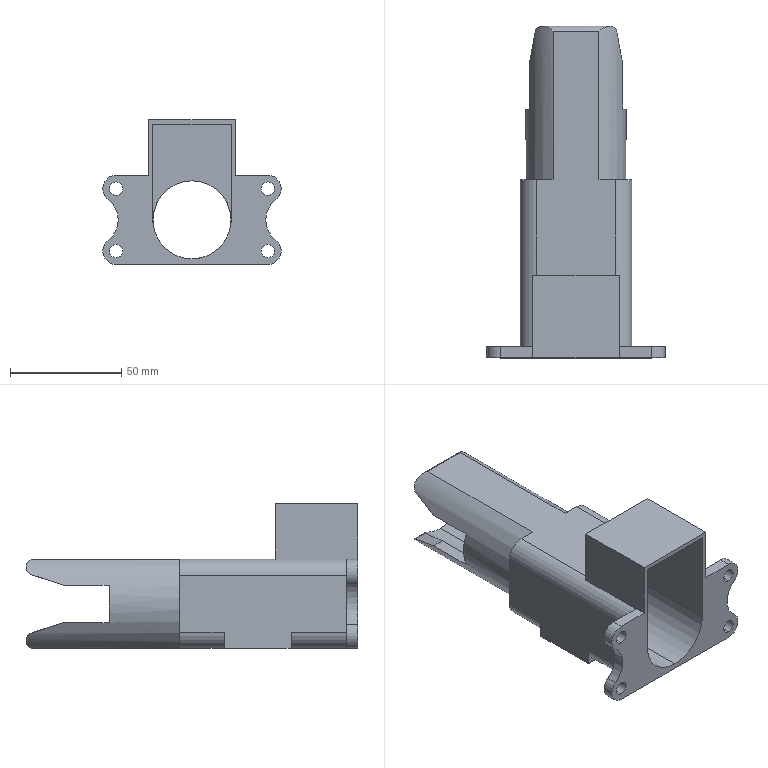Part | SolidWorks | features ICE 22, Extrusion 1, Helix 1, SweepCut 1 | 1 solid | 63 faces | box 80 x 148.861 x 65 mm | volume 115092 mm3 | plane 37 | cylinder 26 | commonest cylinder face diameters 6 x8 16 x6 12 x4 7.559 x2 23.271 x2 35 x2